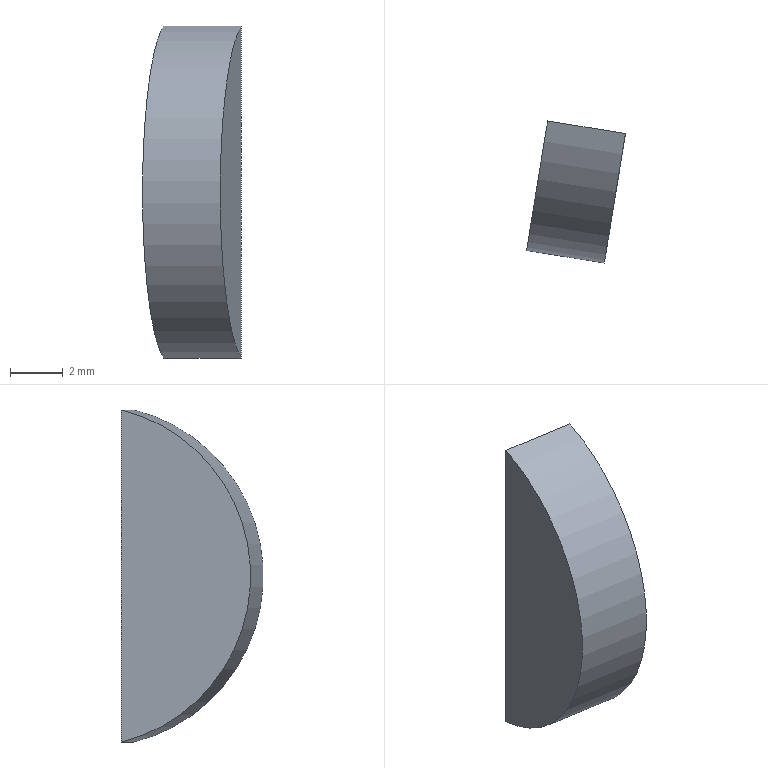Part | SolidWorks | features BaseBody 1 | 1 solid | 4 faces | box 3.765 x 5.417 x 12.649 mm | volume 141.122 mm3 | plane 3 | cylinder 1 | commonest cylinder face diameters 13 x1
STEP:
#1=CARTESIAN_POINT('',(385.524,108.048,50.5));
#2=VERTEX_POINT('',#1);
#3=CARTESIAN_POINT('',(385.524,108.048,63.149));
#4=VERTEX_POINT('',#3);
#5=CARTESIAN_POINT('',(385.765,109.529,56.825));
#6=DIRECTION('',(-0.987,0.1608,0.));
#7=DIRECTION('',(0.,0.,-1.));
#8=AXIS2_PLACEMENT_3D('',#5,#6,#7);
#9=CIRCLE('',#8,6.5);
#10=EDGE_CURVE('',#2,#4,#9,.T.);
#11=ORIENTED_EDGE('',*,*,#10,.T.);
#12=CARTESIAN_POINT('',(382.563,108.531,63.149));
#13=VERTEX_POINT('',#12);
#14=CARTESIAN_POINT('',(382.563,108.531,63.149));
#15=DIRECTION('',(0.987,-0.1608,0.));
#16=VECTOR('',#15,1000.);
#17=LINE('',#14,#16);
#18=EDGE_CURVE('',#13,#4,#17,.T.);
#19=ORIENTED_EDGE('',*,*,#18,.F.);
#20=CARTESIAN_POINT('',(382.563,108.531,50.5));
#21=VERTEX_POINT('',#20);
#22=CARTESIAN_POINT('',(382.804,110.011,56.825));
#23=DIRECTION('',(-0.987,0.1608,0.));
#24=DIRECTION('',(0.,0.,-1.));
#25=AXIS2_PLACEMENT_3D('',#22,#23,#24);
#26=CIRCLE('',#25,6.5);
#27=EDGE_CURVE('',#21,#13,#26,.T.);
#28=ORIENTED_EDGE('',*,*,#27,.F.);
#29=CARTESIAN_POINT('',(382.563,108.531,50.5));
#30=DIRECTION('',(0.987,-0.1608,0.));
#31=VECTOR('',#30,1000.);
#32=LINE('',#29,#31);
#33=EDGE_CURVE('',#21,#2,#32,.T.);
#34=ORIENTED_EDGE('',*,*,#33,.T.);
#35=EDGE_LOOP('',(#11,#19,#28,#34));
#36=FACE_OUTER_BOUND('',#35,.T.);
#37=CARTESIAN_POINT('',(382.804,110.011,56.825));
#38=DIRECTION('',(0.987,-0.1608,0.));
#39=DIRECTION('',(0.,0.,1.));
#40=AXIS2_PLACEMENT_3D('',#37,#38,#39);
#41=CYLINDRICAL_SURFACE('',#40,6.5);
#42=ADVANCED_FACE('',(#36),#41,.T.);
#43=CARTESIAN_POINT('',(385.524,108.048,63.149));
#44=DIRECTION('',(0.,0.,-1.));
#45=VECTOR('',#44,1000.);
#46=LINE('',#43,#45);
#47=EDGE_CURVE('',#4,#2,#46,.T.);
#48=ORIENTED_EDGE('',*,*,#47,.T.);
#49=ORIENTED_EDGE('',*,*,#33,.F.);
#50=CARTESIAN_POINT('',(382.563,108.531,63.149));
#51=DIRECTION('',(0.,0.,-1.));
#52=VECTOR('',#51,1000.);
#53=LINE('',#50,#52);
#54=EDGE_CURVE('',#13,#21,#53,.T.);
#55=ORIENTED_EDGE('',*,*,#54,.F.);
#56=ORIENTED_EDGE('',*,*,#18,.T.);
#57=EDGE_LOOP('',(#48,#49,#55,#56));
#58=FACE_OUTER_BOUND('',#57,.T.);
#59=CARTESIAN_POINT('',(382.563,108.531,63.149));
#60=DIRECTION('',(-0.1608,-0.987,0.));
#61=DIRECTION('',(-0.987,0.1608,0.));
#62=AXIS2_PLACEMENT_3D('',#59,#60,#61);
#63=PLANE('',#62);
#64=ADVANCED_FACE('',(#58),#63,.F.);
#65=ORIENTED_EDGE('',*,*,#27,.T.);
#66=ORIENTED_EDGE('',*,*,#54,.T.);
#67=EDGE_LOOP('',(#65,#66));
#68=FACE_OUTER_BOUND('',#67,.T.);
#69=CARTESIAN_POINT('',(382.804,110.011,56.825));
#70=DIRECTION('',(-0.987,0.1608,0.));
#71=DIRECTION('',(0.,0.,-1.));
#72=AXIS2_PLACEMENT_3D('',#69,#70,#71);
#73=PLANE('',#72);
#74=ADVANCED_FACE('',(#68),#73,.T.);
#75=ORIENTED_EDGE('',*,*,#10,.F.);
#76=ORIENTED_EDGE('',*,*,#47,.F.);
#77=EDGE_LOOP('',(#75,#76));
#78=FACE_OUTER_BOUND('',#77,.T.);
#79=CARTESIAN_POINT('',(385.765,109.529,56.825));
#80=DIRECTION('',(-0.987,0.1608,0.));
#81=DIRECTION('',(0.,0.,-1.));
#82=AXIS2_PLACEMENT_3D('',#79,#80,#81);
#83=PLANE('',#82);
#84=ADVANCED_FACE('',(#78),#83,.F.);
#85=CLOSED_SHELL('',(#42,#64,#74,#84));
#86=MANIFOLD_SOLID_BREP('',#85);
#87=CARTESIAN_POINT('',(0.,0.,0.));
#88=DIRECTION('',(0.,0.,1.));
#89=DIRECTION('',(1.,0.,0.));
#90=AXIS2_PLACEMENT_3D('',#87,#88,#89);
#91=(LENGTH_UNIT()NAMED_UNIT(*)SI_UNIT(.MILLI.,.METRE.));
#92=UNCERTAINTY_MEASURE_WITH_UNIT(LENGTH_MEASURE(0.00001),#91,'','');
#93=(NAMED_UNIT(*)PLANE_ANGLE_UNIT()SI_UNIT($,.RADIAN.));
#94=(NAMED_UNIT(*)SI_UNIT($,.STERADIAN.)SOLID_ANGLE_UNIT());
#95=(GEOMETRIC_REPRESENTATION_CONTEXT(3)GLOBAL_UNCERTAINTY_ASSIGNED_CONTEXT((#92))GLOBAL_UNIT_ASSIGNED_CONTEXT((#91,#93,#94))REPRESENTATION_CONTEXT('',''));
#96=ADVANCED_BREP_SHAPE_REPRESENTATION('',(#86,#90),#95);